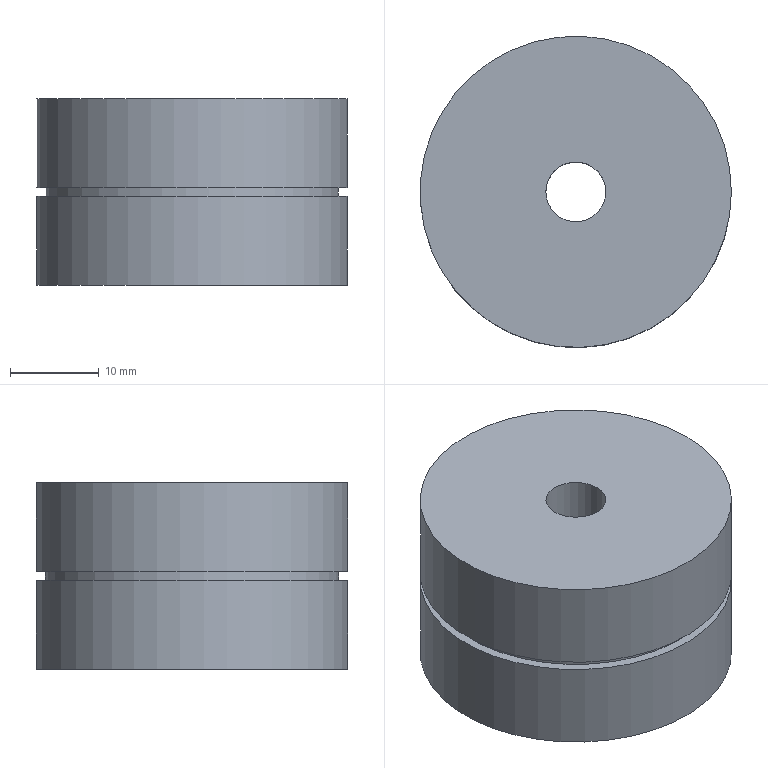Part | NX | features BREP 1, DATUM_CSYS 1 | 1 solid | 8 faces | box 35 x 35 x 21 mm | volume 19346 mm3 | plane 4 | cylinder 4 | commonest cylinder face diameters 35 x2 6.75 x1 33 x1
STEP:
#1=CARTESIAN_POINT('',(17.5,0.,0.));
#2=VERTEX_POINT('',#1);
#3=CARTESIAN_POINT('',(0.,0.,0.));
#4=DIRECTION('',(0.,0.,1.));
#5=DIRECTION('',(1.,0.,0.));
#6=AXIS2_PLACEMENT_3D('',#3,#4,#5);
#7=CIRCLE('',#6,17.5);
#8=EDGE_CURVE('',#2,#2,#7,.T.);
#9=ORIENTED_EDGE('',*,*,#8,.F.);
#10=EDGE_LOOP('',(#9));
#11=FACE_BOUND('',#10,.T.);
#12=CARTESIAN_POINT('',(3.375,0.,0.));
#13=VERTEX_POINT('',#12);
#14=CARTESIAN_POINT('',(0.,0.,0.));
#15=DIRECTION('',(0.,0.,-1.));
#16=DIRECTION('',(1.,0.,0.));
#17=AXIS2_PLACEMENT_3D('',#14,#15,#16);
#18=CIRCLE('',#17,3.375);
#19=EDGE_CURVE('',#13,#13,#18,.T.);
#20=ORIENTED_EDGE('',*,*,#19,.F.);
#21=EDGE_LOOP('',(#20));
#22=FACE_BOUND('',#21,.T.);
#23=CARTESIAN_POINT('',(0.,0.,0.));
#24=DIRECTION('',(0.,0.,1.));
#25=DIRECTION('',(-1.,0.,0.));
#26=AXIS2_PLACEMENT_3D('',#23,#24,#25);
#27=PLANE('',#26);
#28=ADVANCED_FACE('',(#11,#22),#27,.F.);
#29=CARTESIAN_POINT('',(17.5,0.,21.));
#30=VERTEX_POINT('',#29);
#31=CARTESIAN_POINT('',(0.,0.,21.));
#32=DIRECTION('',(0.,0.,1.));
#33=DIRECTION('',(1.,0.,0.));
#34=AXIS2_PLACEMENT_3D('',#31,#32,#33);
#35=CIRCLE('',#34,17.5);
#36=EDGE_CURVE('',#30,#30,#35,.T.);
#37=ORIENTED_EDGE('',*,*,#36,.T.);
#38=EDGE_LOOP('',(#37));
#39=FACE_BOUND('',#38,.T.);
#40=CARTESIAN_POINT('',(3.375,0.,21.));
#41=VERTEX_POINT('',#40);
#42=CARTESIAN_POINT('',(0.,0.,21.));
#43=DIRECTION('',(0.,0.,-1.));
#44=DIRECTION('',(1.,0.,0.));
#45=AXIS2_PLACEMENT_3D('',#42,#43,#44);
#46=CIRCLE('',#45,3.375);
#47=EDGE_CURVE('',#41,#41,#46,.T.);
#48=ORIENTED_EDGE('',*,*,#47,.T.);
#49=EDGE_LOOP('',(#48));
#50=FACE_BOUND('',#49,.T.);
#51=CARTESIAN_POINT('',(0.,0.,21.));
#52=DIRECTION('',(0.,0.,1.));
#53=DIRECTION('',(-1.,0.,0.));
#54=AXIS2_PLACEMENT_3D('',#51,#52,#53);
#55=PLANE('',#54);
#56=ADVANCED_FACE('',(#39,#50),#55,.T.);
#57=ORIENTED_EDGE('',*,*,#8,.T.);
#58=CARTESIAN_POINT('',(17.5,0.,10.));
#59=VERTEX_POINT('',#58);
#60=CARTESIAN_POINT('',(17.5,0.,0.));
#61=DIRECTION('',(0.,0.,1.));
#62=VECTOR('',#61,1000.);
#63=LINE('',#60,#62);
#64=EDGE_CURVE('',#2,#59,#63,.T.);
#65=ORIENTED_EDGE('',*,*,#64,.T.);
#66=CARTESIAN_POINT('',(0.,0.,10.));
#67=DIRECTION('',(0.,0.,1.));
#68=DIRECTION('',(1.,0.,0.));
#69=AXIS2_PLACEMENT_3D('',#66,#67,#68);
#70=CIRCLE('',#69,17.5);
#71=EDGE_CURVE('',#59,#59,#70,.T.);
#72=ORIENTED_EDGE('',*,*,#71,.F.);
#73=ORIENTED_EDGE('',*,*,#64,.F.);
#74=EDGE_LOOP('',(#57,#65,#72,#73));
#75=FACE_BOUND('',#74,.T.);
#76=CARTESIAN_POINT('',(0.,0.,0.));
#77=DIRECTION('',(0.,0.,1.));
#78=DIRECTION('',(-1.,0.,0.));
#79=AXIS2_PLACEMENT_3D('',#76,#77,#78);
#80=CYLINDRICAL_SURFACE('',#79,17.5);
#81=ADVANCED_FACE('',(#75),#80,.T.);
#82=ORIENTED_EDGE('',*,*,#36,.F.);
#83=CARTESIAN_POINT('',(17.5,0.,11.));
#84=VERTEX_POINT('',#83);
#85=CARTESIAN_POINT('',(17.5,0.,11.));
#86=DIRECTION('',(0.,0.,1.));
#87=VECTOR('',#86,1000.);
#88=LINE('',#85,#87);
#89=EDGE_CURVE('',#84,#30,#88,.T.);
#90=ORIENTED_EDGE('',*,*,#89,.F.);
#91=CARTESIAN_POINT('',(0.,0.,11.));
#92=DIRECTION('',(0.,0.,-1.));
#93=DIRECTION('',(1.,0.,0.));
#94=AXIS2_PLACEMENT_3D('',#91,#92,#93);
#95=CIRCLE('',#94,17.5);
#96=EDGE_CURVE('',#84,#84,#95,.T.);
#97=ORIENTED_EDGE('',*,*,#96,.F.);
#98=ORIENTED_EDGE('',*,*,#89,.T.);
#99=EDGE_LOOP('',(#82,#90,#97,#98));
#100=FACE_BOUND('',#99,.T.);
#101=CARTESIAN_POINT('',(0.,0.,0.));
#102=DIRECTION('',(0.,0.,1.));
#103=DIRECTION('',(-1.,0.,0.));
#104=AXIS2_PLACEMENT_3D('',#101,#102,#103);
#105=CYLINDRICAL_SURFACE('',#104,17.5);
#106=ADVANCED_FACE('',(#100),#105,.T.);
#107=ORIENTED_EDGE('',*,*,#71,.T.);
#108=EDGE_LOOP('',(#107));
#109=FACE_BOUND('',#108,.T.);
#110=CARTESIAN_POINT('',(16.5,0.,10.));
#111=VERTEX_POINT('',#110);
#112=CARTESIAN_POINT('',(0.,0.,10.));
#113=DIRECTION('',(0.,0.,-1.));
#114=DIRECTION('',(1.,0.,0.));
#115=AXIS2_PLACEMENT_3D('',#112,#113,#114);
#116=CIRCLE('',#115,16.5);
#117=EDGE_CURVE('',#111,#111,#116,.T.);
#118=ORIENTED_EDGE('',*,*,#117,.T.);
#119=EDGE_LOOP('',(#118));
#120=FACE_BOUND('',#119,.T.);
#121=CARTESIAN_POINT('',(0.,0.,10.));
#122=DIRECTION('',(0.,0.,-1.));
#123=DIRECTION('',(-1.,0.,0.));
#124=AXIS2_PLACEMENT_3D('',#121,#122,#123);
#125=PLANE('',#124);
#126=ADVANCED_FACE('',(#109,#120),#125,.F.);
#127=CARTESIAN_POINT('',(16.5,0.,11.));
#128=VERTEX_POINT('',#127);
#129=CARTESIAN_POINT('',(0.,0.,11.));
#130=DIRECTION('',(0.,0.,-1.));
#131=DIRECTION('',(1.,0.,0.));
#132=AXIS2_PLACEMENT_3D('',#129,#130,#131);
#133=CIRCLE('',#132,16.5);
#134=EDGE_CURVE('',#128,#128,#133,.T.);
#135=ORIENTED_EDGE('',*,*,#134,.T.);
#136=CARTESIAN_POINT('',(16.5,0.,11.));
#137=DIRECTION('',(0.,0.,-1.));
#138=VECTOR('',#137,1000.);
#139=LINE('',#136,#138);
#140=EDGE_CURVE('',#128,#111,#139,.T.);
#141=ORIENTED_EDGE('',*,*,#140,.T.);
#142=ORIENTED_EDGE('',*,*,#117,.F.);
#143=ORIENTED_EDGE('',*,*,#140,.F.);
#144=EDGE_LOOP('',(#135,#141,#142,#143));
#145=FACE_BOUND('',#144,.T.);
#146=CARTESIAN_POINT('',(0.,0.,11.));
#147=DIRECTION('',(0.,0.,-1.));
#148=DIRECTION('',(-1.,0.,0.));
#149=AXIS2_PLACEMENT_3D('',#146,#147,#148);
#150=CYLINDRICAL_SURFACE('',#149,16.5);
#151=ADVANCED_FACE('',(#145),#150,.T.);
#152=ORIENTED_EDGE('',*,*,#96,.T.);
#153=EDGE_LOOP('',(#152));
#154=FACE_BOUND('',#153,.T.);
#155=ORIENTED_EDGE('',*,*,#134,.F.);
#156=EDGE_LOOP('',(#155));
#157=FACE_BOUND('',#156,.T.);
#158=CARTESIAN_POINT('',(0.,0.,11.));
#159=DIRECTION('',(0.,0.,1.));
#160=DIRECTION('',(-1.,0.,0.));
#161=AXIS2_PLACEMENT_3D('',#158,#159,#160);
#162=PLANE('',#161);
#163=ADVANCED_FACE('',(#154,#157),#162,.F.);
#164=CARTESIAN_POINT('',(3.375,0.,21.));
#165=DIRECTION('',(0.,0.,-1.));
#166=VECTOR('',#165,1000.);
#167=LINE('',#164,#166);
#168=EDGE_CURVE('',#41,#13,#167,.T.);
#169=ORIENTED_EDGE('',*,*,#168,.T.);
#170=ORIENTED_EDGE('',*,*,#19,.T.);
#171=ORIENTED_EDGE('',*,*,#168,.F.);
#172=ORIENTED_EDGE('',*,*,#47,.F.);
#173=EDGE_LOOP('',(#169,#170,#171,#172));
#174=FACE_BOUND('',#173,.T.);
#175=CARTESIAN_POINT('',(0.,0.,21.));
#176=DIRECTION('',(0.,0.,-1.));
#177=DIRECTION('',(-1.,0.,0.));
#178=AXIS2_PLACEMENT_3D('',#175,#176,#177);
#179=CYLINDRICAL_SURFACE('',#178,3.375);
#180=ADVANCED_FACE('',(#174),#179,.F.);
#181=CLOSED_SHELL('',(#28,#56,#81,#106,#126,#151,#163,#180));
#182=MANIFOLD_SOLID_BREP('',#181);
#183=(LENGTH_UNIT()NAMED_UNIT(*)SI_UNIT(.MILLI.,.METRE.));
#184=UNCERTAINTY_MEASURE_WITH_UNIT(LENGTH_MEASURE(0.00001),#183,'','');
#185=(NAMED_UNIT(*)PLANE_ANGLE_UNIT()SI_UNIT($,.RADIAN.));
#186=(NAMED_UNIT(*)SI_UNIT($,.STERADIAN.)SOLID_ANGLE_UNIT());
#187=(GEOMETRIC_REPRESENTATION_CONTEXT(3)GLOBAL_UNCERTAINTY_ASSIGNED_CONTEXT((#184))GLOBAL_UNIT_ASSIGNED_CONTEXT((#183,#185,#186))REPRESENTATION_CONTEXT('',''));
#188=ADVANCED_BREP_SHAPE_REPRESENTATION('',(#182),#187);